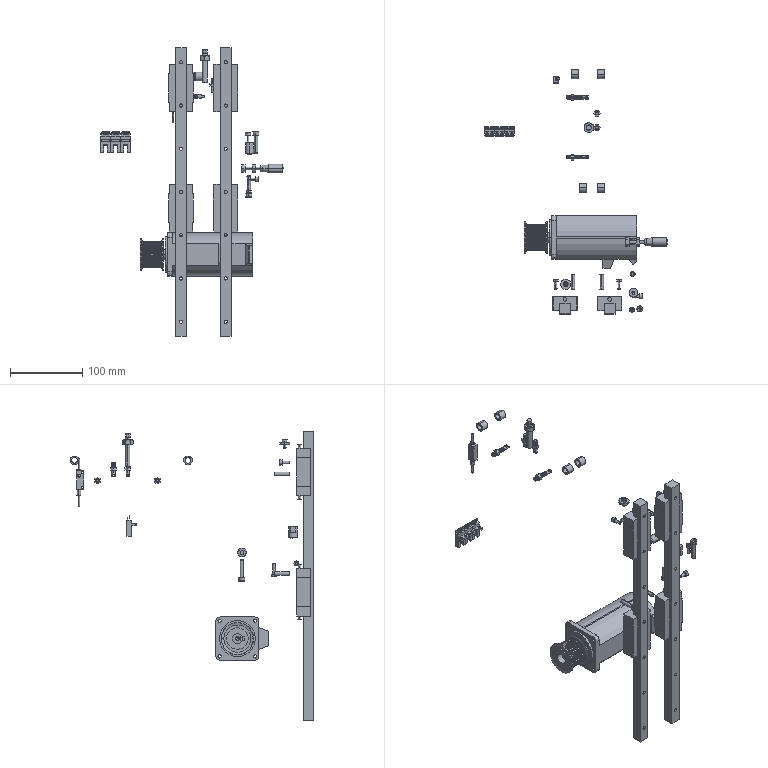Part | NX | 45 solids | 2676 faces | box 253.4 x 338.05 x 400 mm | volume 730031 mm3 | plane 1757 | cylinder 725 | cone 140 | spline 44 | sphere 6 | torus 4 | commonest cylinder face diameters 5 x203 0.5 x52 6.55 x52 1.1 x48 37.24 x48 4.5 x36